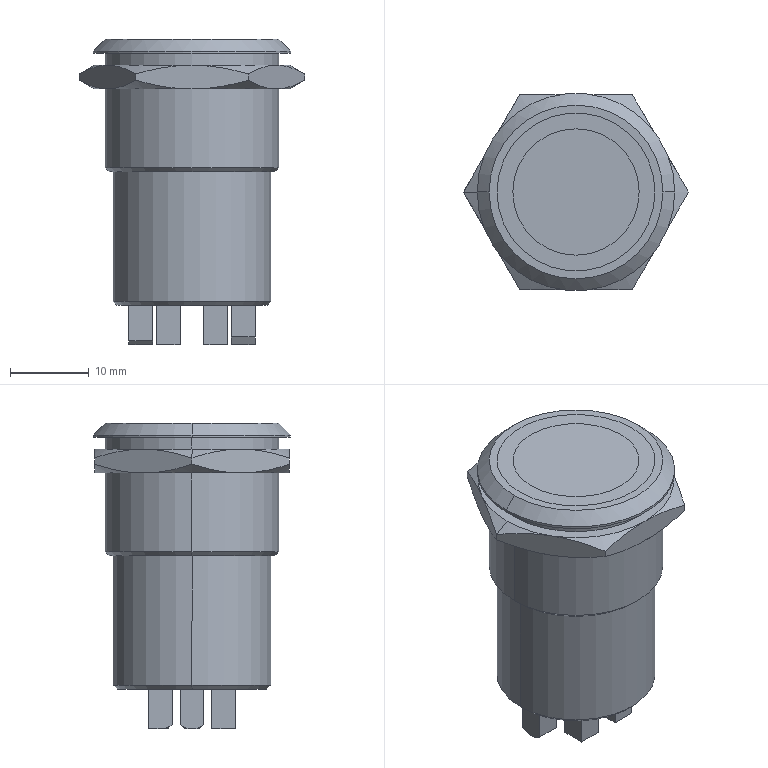Part | STEP file | Metal push button switch ring light GQ22-L-11E_G_24V_S | 2 solids | 88 faces | box 28.5 x 25 x 38.7 mm | volume 12469 mm3 | plane 52 | cone 20 | cylinder 16 | commonest cylinder face diameters 20 x6 16 x4 22 x4 25 x2